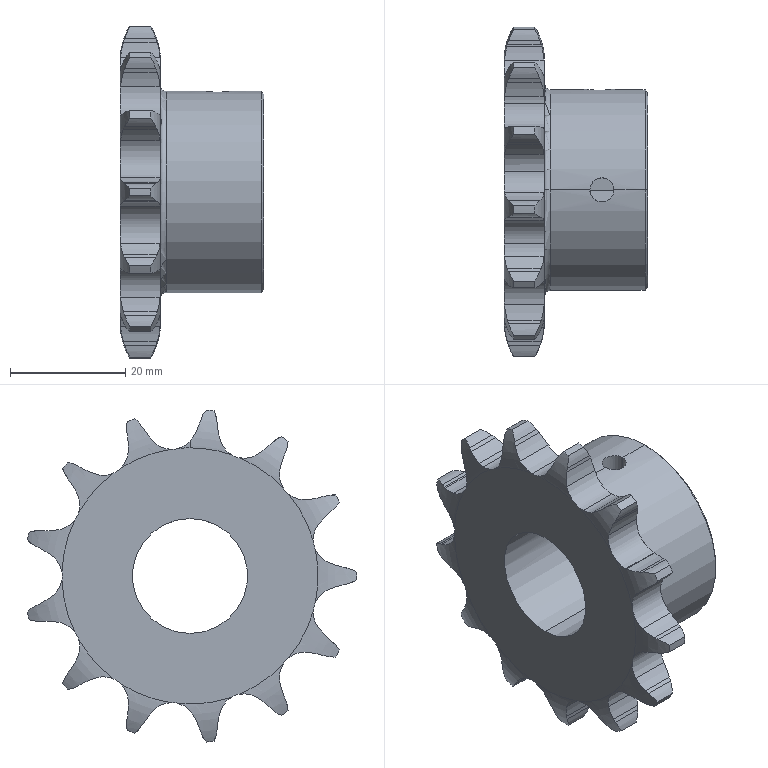Part | SolidWorks | features HoleWzd 2, Chamfer 1, CirPattern 1, Cut 1, Fillet 1, ICE 1, Revolution 1 | 1 solid | 154 faces | box 25.008 x 57.316 x 57.728 mm | volume 22409 mm3 | cylinder 93 | torus 30 | plane 29 | cone 2 | commonest cylinder face diameters 12.597 x28 22.269 x27 8.653 x17 58 x13 4.2 x4 20 x2